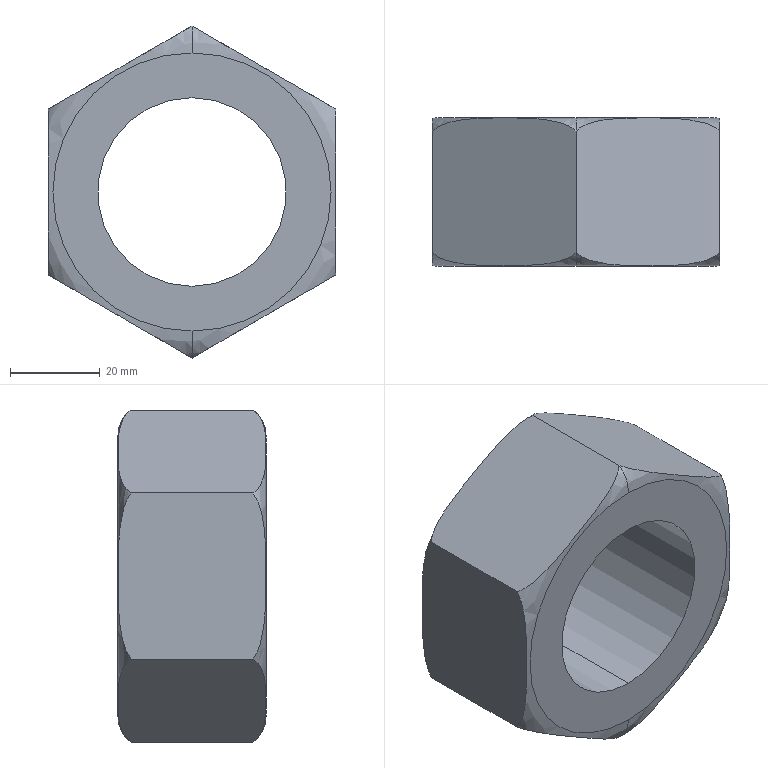Part | SolidWorks | features Extrusion 1, RevCut 1 | 1 solid | 14 faces | box 64 x 33 x 73.901 mm | volume 71017 mm3 | plane 8 | spline 4 | cylinder 2 | commonest cylinder face diameters 42 x2
STEP:
#1=CARTESIAN_POINT('',(0.,13.5,-36.95));
#2=VERTEX_POINT('',#1);
#3=CARTESIAN_POINT('',(32.,13.5,-18.475));
#4=VERTEX_POINT('',#3);
#5=CARTESIAN_POINT('',(0.,13.5,-36.95));
#6=CARTESIAN_POINT('',(0.5345,14.021,-36.642));
#7=CARTESIAN_POINT('',(1.133,14.41,-36.297));
#8=CARTESIAN_POINT('',(2.082,14.885,-35.749));
#9=CARTESIAN_POINT('',(2.409,15.025,-35.56));
#10=CARTESIAN_POINT('',(3.065,15.271,-35.181));
#11=CARTESIAN_POINT('',(3.395,15.377,-34.99));
#12=CARTESIAN_POINT('',(4.392,15.661,-34.414));
#13=CARTESIAN_POINT('',(5.064,15.802,-34.026));
#14=CARTESIAN_POINT('',(6.417,16.026,-33.246));
#15=CARTESIAN_POINT('',(7.097,16.109,-32.853));
#16=CARTESIAN_POINT('',(8.464,16.239,-32.064));
#17=CARTESIAN_POINT('',(9.15,16.285,-31.668));
#18=CARTESIAN_POINT('',(10.522,16.356,-30.876));
#19=CARTESIAN_POINT('',(11.207,16.38,-30.48));
#20=CARTESIAN_POINT('',(13.265,16.433,-29.292));
#21=CARTESIAN_POINT('',(14.637,16.443,-28.5));
#22=CARTESIAN_POINT('',(17.381,16.443,-26.915));
#23=CARTESIAN_POINT('',(18.753,16.432,-26.123));
#24=CARTESIAN_POINT('',(21.498,16.362,-24.538));
#25=CARTESIAN_POINT('',(22.87,16.303,-23.747));
#26=CARTESIAN_POINT('',(24.92,16.107,-22.563));
#27=CARTESIAN_POINT('',(25.603,16.023,-22.169));
#28=CARTESIAN_POINT('',(26.963,15.796,-21.383));
#29=CARTESIAN_POINT('',(27.638,15.654,-20.994));
#30=CARTESIAN_POINT('',(28.969,15.272,-20.225));
#31=CARTESIAN_POINT('',(29.629,15.031,-19.844));
#32=CARTESIAN_POINT('',(30.564,14.561,-19.304));
#33=CARTESIAN_POINT('',(30.868,14.385,-19.129));
#34=CARTESIAN_POINT('',(31.452,13.984,-18.791));
#35=CARTESIAN_POINT('',(31.734,13.759,-18.629));
#36=CARTESIAN_POINT('',(32.,13.5,-18.475));
#37=B_SPLINE_CURVE_WITH_KNOTS('',3,(#5,#6,#7,#8,#9,#10,#11,#12,#13,#14,#15,#16,#17,#18,#19,#20,#21,#22,#23,#24,#25,#26,#27,#28,#29,#30,#31,#32,#33,#34,#35,#36),.UNSPECIFIED.,.F.,.F.,(4,2,2,2,2,2,2,2,2,2,2,2,2,2,2,4),(0.,0.002378,0.003566,0.004755,0.007133,0.009511,0.01189,0.01427,0.01902,0.02378,0.02853,0.03091,0.03329,0.03566,0.03685,0.03804),.UNSPECIFIED.);
#38=EDGE_CURVE('',#2,#4,#37,.T.);
#39=ORIENTED_EDGE('',*,*,#38,.F.);
#40=CARTESIAN_POINT('',(0.,16.5,-30.95));
#41=VERTEX_POINT('',#40);
#42=CARTESIAN_POINT('',(0.,13.5,-36.95));
#43=CARTESIAN_POINT('',(0.,15.629,-35.689));
#44=CARTESIAN_POINT('',(0.,16.5,-33.372));
#45=CARTESIAN_POINT('',(0.,16.5,-30.95));
#46=B_SPLINE_CURVE_WITH_KNOTS('',3,(#42,#43,#44,#45),.UNSPECIFIED.,.F.,.F.,(4,4),(0.,1.),.UNSPECIFIED.);
#47=EDGE_CURVE('',#2,#41,#46,.T.);
#48=ORIENTED_EDGE('',*,*,#47,.T.);
#49=CARTESIAN_POINT('',(0.,16.5,30.95));
#50=VERTEX_POINT('',#49);
#51=CARTESIAN_POINT('',(0.,16.5,0.));
#52=DIRECTION('',(0.,1.,0.));
#53=DIRECTION('',(0.,0.,1.));
#54=AXIS2_PLACEMENT_3D('',#51,#52,#53);
#55=CIRCLE('',#54,30.95);
#56=EDGE_CURVE('',#50,#41,#55,.T.);
#57=ORIENTED_EDGE('',*,*,#56,.F.);
#58=CARTESIAN_POINT('',(0.,13.5,36.95));
#59=VERTEX_POINT('',#58);
#60=CARTESIAN_POINT('',(0.,13.5,36.95));
#61=CARTESIAN_POINT('',(0.,15.629,35.689));
#62=CARTESIAN_POINT('',(0.,16.5,33.372));
#63=CARTESIAN_POINT('',(0.,16.5,30.95));
#64=B_SPLINE_CURVE_WITH_KNOTS('',3,(#60,#61,#62,#63),.UNSPECIFIED.,.F.,.F.,(4,4),(0.,1.),.UNSPECIFIED.);
#65=EDGE_CURVE('',#59,#50,#64,.T.);
#66=ORIENTED_EDGE('',*,*,#65,.F.);
#67=CARTESIAN_POINT('',(32.,13.5,18.475));
#68=VERTEX_POINT('',#67);
#69=CARTESIAN_POINT('',(32.,13.5,18.475));
#70=CARTESIAN_POINT('',(31.465,14.021,18.784));
#71=CARTESIAN_POINT('',(30.867,14.41,19.129));
#72=CARTESIAN_POINT('',(29.918,14.885,19.677));
#73=CARTESIAN_POINT('',(29.591,15.025,19.866));
#74=CARTESIAN_POINT('',(28.935,15.271,20.245));
#75=CARTESIAN_POINT('',(28.605,15.377,20.436));
#76=CARTESIAN_POINT('',(27.608,15.661,21.011));
#77=CARTESIAN_POINT('',(26.936,15.802,21.399));
#78=CARTESIAN_POINT('',(25.583,16.026,22.18));
#79=CARTESIAN_POINT('',(24.903,16.109,22.573));
#80=CARTESIAN_POINT('',(23.536,16.239,23.362));
#81=CARTESIAN_POINT('',(22.85,16.285,23.758));
#82=CARTESIAN_POINT('',(21.478,16.356,24.55));
#83=CARTESIAN_POINT('',(20.793,16.38,24.946));
#84=CARTESIAN_POINT('',(18.735,16.433,26.134));
#85=CARTESIAN_POINT('',(17.363,16.443,26.926));
#86=CARTESIAN_POINT('',(14.619,16.443,28.51));
#87=CARTESIAN_POINT('',(13.247,16.432,29.303));
#88=CARTESIAN_POINT('',(10.502,16.362,30.887));
#89=CARTESIAN_POINT('',(9.13,16.303,31.679));
#90=CARTESIAN_POINT('',(7.08,16.107,32.863));
#91=CARTESIAN_POINT('',(6.397,16.023,33.257));
#92=CARTESIAN_POINT('',(5.037,15.796,34.042));
#93=CARTESIAN_POINT('',(4.362,15.654,34.432));
#94=CARTESIAN_POINT('',(3.031,15.272,35.201));
#95=CARTESIAN_POINT('',(2.371,15.031,35.582));
#96=CARTESIAN_POINT('',(1.436,14.561,36.122));
#97=CARTESIAN_POINT('',(1.132,14.385,36.297));
#98=CARTESIAN_POINT('',(0.5476,13.984,36.634));
#99=CARTESIAN_POINT('',(0.2662,13.759,36.797));
#100=CARTESIAN_POINT('',(0.,13.5,36.95));
#101=B_SPLINE_CURVE_WITH_KNOTS('',3,(#69,#70,#71,#72,#73,#74,#75,#76,#77,#78,#79,#80,#81,#82,#83,#84,#85,#86,#87,#88,#89,#90,#91,#92,#93,#94,#95,#96,#97,#98,#99,#100),.UNSPECIFIED.,.F.,.F.,(4,2,2,2,2,2,2,2,2,2,2,2,2,2,2,4),(0.,0.002378,0.003566,0.004755,0.007133,0.009511,0.01189,0.01427,0.01902,0.02378,0.02853,0.03091,0.03329,0.03566,0.03685,0.03804),.UNSPECIFIED.);
#102=EDGE_CURVE('',#68,#59,#101,.T.);
#103=ORIENTED_EDGE('',*,*,#102,.F.);
#104=CARTESIAN_POINT('',(32.,13.5,-18.475));
#105=CARTESIAN_POINT('',(32.,14.021,-17.858));
#106=CARTESIAN_POINT('',(32.,14.41,-17.167));
#107=CARTESIAN_POINT('',(32.,14.885,-16.071));
#108=CARTESIAN_POINT('',(32.,15.025,-15.694));
#109=CARTESIAN_POINT('',(32.,15.271,-14.936));
#110=CARTESIAN_POINT('',(32.,15.377,-14.555));
#111=CARTESIAN_POINT('',(32.,15.661,-13.403));
#112=CARTESIAN_POINT('',(32.,15.802,-12.627));
#113=CARTESIAN_POINT('',(32.,16.026,-11.066));
#114=CARTESIAN_POINT('',(32.,16.109,-10.28));
#115=CARTESIAN_POINT('',(32.,16.239,-8.702));
#116=CARTESIAN_POINT('',(32.,16.285,-7.909));
#117=CARTESIAN_POINT('',(32.,16.356,-6.326));
#118=CARTESIAN_POINT('',(32.,16.38,-5.534));
#119=CARTESIAN_POINT('',(32.,16.433,-3.158));
#120=CARTESIAN_POINT('',(32.,16.443,-1.574));
#121=CARTESIAN_POINT('',(32.,16.443,1.595));
#122=CARTESIAN_POINT('',(32.,16.432,3.179));
#123=CARTESIAN_POINT('',(32.,16.362,6.349));
#124=CARTESIAN_POINT('',(32.,16.303,7.932));
#125=CARTESIAN_POINT('',(32.,16.107,10.3));
#126=CARTESIAN_POINT('',(32.,16.023,11.088));
#127=CARTESIAN_POINT('',(32.,15.796,12.659));
#128=CARTESIAN_POINT('',(32.,15.654,13.438));
#129=CARTESIAN_POINT('',(32.,15.272,14.976));
#130=CARTESIAN_POINT('',(32.,15.031,15.738));
#131=CARTESIAN_POINT('',(32.,14.561,16.818));
#132=CARTESIAN_POINT('',(32.,14.385,17.168));
#133=CARTESIAN_POINT('',(32.,13.984,17.843));
#134=CARTESIAN_POINT('',(32.,13.759,18.168));
#135=CARTESIAN_POINT('',(32.,13.5,18.475));
#136=B_SPLINE_CURVE_WITH_KNOTS('',3,(#104,#105,#106,#107,#108,#109,#110,#111,#112,#113,#114,#115,#116,#117,#118,#119,#120,#121,#122,#123,#124,#125,#126,#127,#128,#129,#130,#131,#132,#133,#134,#135),.UNSPECIFIED.,.F.,.F.,(4,2,2,2,2,2,2,2,2,2,2,2,2,2,2,4),(0.,0.002378,0.003566,0.004755,0.007133,0.009511,0.01189,0.01427,0.01902,0.02378,0.02853,0.03091,0.03329,0.03566,0.03685,0.03804),.UNSPECIFIED.);
#137=EDGE_CURVE('',#4,#68,#136,.T.);
#138=ORIENTED_EDGE('',*,*,#137,.F.);
#139=EDGE_LOOP('',(#39,#48,#57,#66,#103,#138));
#140=FACE_OUTER_BOUND('',#139,.T.);
#141=CARTESIAN_POINT('',(0.,13.5,36.95));
#142=CARTESIAN_POINT('',(73.901,13.5,36.95));
#143=CARTESIAN_POINT('',(73.901,13.5,-36.95));
#144=CARTESIAN_POINT('',(0.,13.5,-36.95));
#145=CARTESIAN_POINT('',(0.,15.629,35.689));
#146=CARTESIAN_POINT('',(71.378,15.629,35.689));
#147=CARTESIAN_POINT('',(71.378,15.629,-35.689));
#148=CARTESIAN_POINT('',(0.,15.629,-35.689));
#149=CARTESIAN_POINT('',(0.,16.5,33.372));
#150=CARTESIAN_POINT('',(66.744,16.5,33.372));
#151=CARTESIAN_POINT('',(66.744,16.5,-33.372));
#152=CARTESIAN_POINT('',(0.,16.5,-33.372));
#153=CARTESIAN_POINT('',(0.,16.5,30.95));
#154=CARTESIAN_POINT('',(61.901,16.5,30.95));
#155=CARTESIAN_POINT('',(61.901,16.5,-30.95));
#156=CARTESIAN_POINT('',(0.,16.5,-30.95));
#157=(BOUNDED_SURFACE()B_SPLINE_SURFACE(3,3,((#141,#142,#143,#144),(#145,#146,#147,#148),(#149,#150,#151,#152),(#153,#154,#155,#156)),.UNSPECIFIED.,.F.,.F.,.F.)B_SPLINE_SURFACE_WITH_KNOTS((4,4),(4,4),(0.,1.),(0.,1.),.UNSPECIFIED.)GEOMETRIC_REPRESENTATION_ITEM()RATIONAL_B_SPLINE_SURFACE(((1.,0.3333,0.3333,1.),(1.,0.3333,0.3333,1.),(1.,0.3333,0.3333,1.),(1.,0.3333,0.3333,1.)))REPRESENTATION_ITEM('')SURFACE());
#158=ADVANCED_FACE('',(#140),#157,.F.);
#159=CARTESIAN_POINT('',(0.,-16.5,30.95));
#160=VERTEX_POINT('',#159);
#161=CARTESIAN_POINT('',(0.,-16.5,-30.95));
#162=VERTEX_POINT('',#161);
#163=CARTESIAN_POINT('',(0.,-16.5,0.));
#164=DIRECTION('',(0.,1.,0.));
#165=DIRECTION('',(0.,0.,1.));
#166=AXIS2_PLACEMENT_3D('',#163,#164,#165);
#167=CIRCLE('',#166,30.95);
#168=EDGE_CURVE('',#160,#162,#167,.T.);
#169=ORIENTED_EDGE('',*,*,#168,.T.);
#170=CARTESIAN_POINT('',(0.,-13.5,-36.95));
#171=VERTEX_POINT('',#170);
#172=CARTESIAN_POINT('',(0.,-16.5,-30.95));
#173=CARTESIAN_POINT('',(0.,-16.5,-33.372));
#174=CARTESIAN_POINT('',(0.,-15.629,-35.689));
#175=CARTESIAN_POINT('',(0.,-13.5,-36.95));
#176=B_SPLINE_CURVE_WITH_KNOTS('',3,(#172,#173,#174,#175),.UNSPECIFIED.,.F.,.F.,(4,4),(0.,1.),.UNSPECIFIED.);
#177=EDGE_CURVE('',#162,#171,#176,.T.);
#178=ORIENTED_EDGE('',*,*,#177,.T.);
#179=CARTESIAN_POINT('',(32.,-13.5,-18.475));
#180=VERTEX_POINT('',#179);
#181=CARTESIAN_POINT('',(32.,-13.5,-18.475));
#182=CARTESIAN_POINT('',(31.465,-14.021,-18.784));
#183=CARTESIAN_POINT('',(30.867,-14.41,-19.129));
#184=CARTESIAN_POINT('',(29.918,-14.885,-19.677));
#185=CARTESIAN_POINT('',(29.591,-15.025,-19.866));
#186=CARTESIAN_POINT('',(28.935,-15.271,-20.245));
#187=CARTESIAN_POINT('',(28.605,-15.377,-20.436));
#188=CARTESIAN_POINT('',(27.608,-15.661,-21.011));
#189=CARTESIAN_POINT('',(26.936,-15.802,-21.399));
#190=CARTESIAN_POINT('',(25.583,-16.026,-22.18));
#191=CARTESIAN_POINT('',(24.903,-16.109,-22.573));
#192=CARTESIAN_POINT('',(23.536,-16.239,-23.362));
#193=CARTESIAN_POINT('',(22.85,-16.285,-23.758));
#194=CARTESIAN_POINT('',(21.478,-16.356,-24.55));
#195=CARTESIAN_POINT('',(20.793,-16.38,-24.946));
#196=CARTESIAN_POINT('',(18.735,-16.433,-26.134));
#197=CARTESIAN_POINT('',(17.363,-16.443,-26.926));
#198=CARTESIAN_POINT('',(14.619,-16.443,-28.51));
#199=CARTESIAN_POINT('',(13.247,-16.432,-29.303));
#200=CARTESIAN_POINT('',(10.502,-16.362,-30.887));
#201=CARTESIAN_POINT('',(9.13,-16.303,-31.679));
#202=CARTESIAN_POINT('',(7.08,-16.107,-32.863));
#203=CARTESIAN_POINT('',(6.397,-16.023,-33.257));
#204=CARTESIAN_POINT('',(5.037,-15.796,-34.042));
#205=CARTESIAN_POINT('',(4.362,-15.654,-34.432));
#206=CARTESIAN_POINT('',(3.031,-15.272,-35.201));
#207=CARTESIAN_POINT('',(2.371,-15.031,-35.582));
#208=CARTESIAN_POINT('',(1.436,-14.561,-36.122));
#209=CARTESIAN_POINT('',(1.132,-14.385,-36.297));
#210=CARTESIAN_POINT('',(0.5476,-13.984,-36.634));
#211=CARTESIAN_POINT('',(0.2662,-13.759,-36.797));
#212=CARTESIAN_POINT('',(0.,-13.5,-36.95));
#213=B_SPLINE_CURVE_WITH_KNOTS('',3,(#181,#182,#183,#184,#185,#186,#187,#188,#189,#190,#191,#192,#193,#194,#195,#196,#197,#198,#199,#200,#201,#202,#203,#204,#205,#206,#207,#208,#209,#210,#211,#212),.UNSPECIFIED.,.F.,.F.,(4,2,2,2,2,2,2,2,2,2,2,2,2,2,2,4),(0.,0.002378,0.003566,0.004755,0.007133,0.009511,0.01189,0.01427,0.01902,0.02378,0.02853,0.03091,0.03329,0.03566,0.03685,0.03804),.UNSPECIFIED.);
#214=EDGE_CURVE('',#180,#171,#213,.T.);
#215=ORIENTED_EDGE('',*,*,#214,.F.);
#216=CARTESIAN_POINT('',(32.,-13.5,18.475));
#217=VERTEX_POINT('',#216);
#218=CARTESIAN_POINT('',(32.,-13.5,18.475));
#219=CARTESIAN_POINT('',(32.,-14.021,17.858));
#220=CARTESIAN_POINT('',(32.,-14.41,17.167));
#221=CARTESIAN_POINT('',(32.,-14.885,16.071));
#222=CARTESIAN_POINT('',(32.,-15.025,15.694));
#223=CARTESIAN_POINT('',(32.,-15.271,14.936));
#224=CARTESIAN_POINT('',(32.,-15.377,14.555));
#225=CARTESIAN_POINT('',(32.,-15.661,13.403));
#226=CARTESIAN_POINT('',(32.,-15.802,12.627));
#227=CARTESIAN_POINT('',(32.,-16.026,11.066));
#228=CARTESIAN_POINT('',(32.,-16.109,10.28));
#229=CARTESIAN_POINT('',(32.,-16.239,8.702));
#230=CARTESIAN_POINT('',(32.,-16.285,7.909));
#231=CARTESIAN_POINT('',(32.,-16.356,6.326));
#232=CARTESIAN_POINT('',(32.,-16.38,5.534));
#233=CARTESIAN_POINT('',(32.,-16.433,3.158));
#234=CARTESIAN_POINT('',(32.,-16.443,1.574));
#235=CARTESIAN_POINT('',(32.,-16.443,-1.595));
#236=CARTESIAN_POINT('',(32.,-16.432,-3.179));
#237=CARTESIAN_POINT('',(32.,-16.362,-6.349));
#238=CARTESIAN_POINT('',(32.,-16.303,-7.932));
#239=CARTESIAN_POINT('',(32.,-16.107,-10.3));
#240=CARTESIAN_POINT('',(32.,-16.023,-11.088));
#241=CARTESIAN_POINT('',(32.,-15.796,-12.659));
#242=CARTESIAN_POINT('',(32.,-15.654,-13.438));
#243=CARTESIAN_POINT('',(32.,-15.272,-14.976));
#244=CARTESIAN_POINT('',(32.,-15.031,-15.738));
#245=CARTESIAN_POINT('',(32.,-14.561,-16.818));
#246=CARTESIAN_POINT('',(32.,-14.385,-17.168));
#247=CARTESIAN_POINT('',(32.,-13.984,-17.843));
#248=CARTESIAN_POINT('',(32.,-13.759,-18.168));
#249=CARTESIAN_POINT('',(32.,-13.5,-18.475));
#250=B_SPLINE_CURVE_WITH_KNOTS('',3,(#218,#219,#220,#221,#222,#223,#224,#225,#226,#227,#228,#229,#230,#231,#232,#233,#234,#235,#236,#237,#238,#239,#240,#241,#242,#243,#244,#245,#246,#247,#248,#249),.UNSPECIFIED.,.F.,.F.,(4,2,2,2,2,2,2,2,2,2,2,2,2,2,2,4),(0.,0.002378,0.003566,0.004755,0.007133,0.009511,0.01189,0.01427,0.01902,0.02378,0.02853,0.03091,0.03329,0.03566,0.03685,0.03804),.UNSPECIFIED.);
#251=EDGE_CURVE('',#217,#180,#250,.T.);
#252=ORIENTED_EDGE('',*,*,#251,.F.);
#253=CARTESIAN_POINT('',(0.,-13.5,36.95));
#254=VERTEX_POINT('',#253);
#255=CARTESIAN_POINT('',(0.,-13.5,36.95));
#256=CARTESIAN_POINT('',(0.5345,-14.021,36.642));
#257=CARTESIAN_POINT('',(1.133,-14.41,36.297));
#258=CARTESIAN_POINT('',(2.082,-14.885,35.749));
#259=CARTESIAN_POINT('',(2.409,-15.025,35.56));
#260=CARTESIAN_POINT('',(3.065,-15.271,35.181));
#261=CARTESIAN_POINT('',(3.395,-15.377,34.99));
#262=CARTESIAN_POINT('',(4.392,-15.661,34.414));
#263=CARTESIAN_POINT('',(5.064,-15.802,34.026));
#264=CARTESIAN_POINT('',(6.417,-16.026,33.246));
#265=CARTESIAN_POINT('',(7.097,-16.109,32.853));
#266=CARTESIAN_POINT('',(8.464,-16.239,32.064));
#267=CARTESIAN_POINT('',(9.15,-16.285,31.668));
#268=CARTESIAN_POINT('',(10.522,-16.356,30.876));
#269=CARTESIAN_POINT('',(11.207,-16.38,30.48));
#270=CARTESIAN_POINT('',(13.265,-16.433,29.292));
#271=CARTESIAN_POINT('',(14.637,-16.443,28.5));
#272=CARTESIAN_POINT('',(17.381,-16.443,26.915));
#273=CARTESIAN_POINT('',(18.753,-16.432,26.123));
#274=CARTESIAN_POINT('',(21.498,-16.362,24.538));
#275=CARTESIAN_POINT('',(22.87,-16.303,23.747));
#276=CARTESIAN_POINT('',(24.92,-16.107,22.563));
#277=CARTESIAN_POINT('',(25.603,-16.023,22.169));
#278=CARTESIAN_POINT('',(26.963,-15.796,21.383));
#279=CARTESIAN_POINT('',(27.638,-15.654,20.994));
#280=CARTESIAN_POINT('',(28.969,-15.272,20.225));
#281=CARTESIAN_POINT('',(29.629,-15.031,19.844));
#282=CARTESIAN_POINT('',(30.564,-14.561,19.304));
#283=CARTESIAN_POINT('',(30.868,-14.385,19.129));
#284=CARTESIAN_POINT('',(31.452,-13.984,18.791));
#285=CARTESIAN_POINT('',(31.734,-13.759,18.629));
#286=CARTESIAN_POINT('',(32.,-13.5,18.475));
#287=B_SPLINE_CURVE_WITH_KNOTS('',3,(#255,#256,#257,#258,#259,#260,#261,#262,#263,#264,#265,#266,#267,#268,#269,#270,#271,#272,#273,#274,#275,#276,#277,#278,#279,#280,#281,#282,#283,#284,#285,#286),.UNSPECIFIED.,.F.,.F.,(4,2,2,2,2,2,2,2,2,2,2,2,2,2,2,4),(0.,0.002378,0.003566,0.004755,0.007133,0.009511,0.01189,0.01427,0.01902,0.02378,0.02853,0.03091,0.03329,0.03566,0.03685,0.03804),.UNSPECIFIED.);
#288=EDGE_CURVE('',#254,#217,#287,.T.);
#289=ORIENTED_EDGE('',*,*,#288,.F.);
#290=CARTESIAN_POINT('',(0.,-16.5,30.95));
#291=CARTESIAN_POINT('',(0.,-16.5,33.372));
#292=CARTESIAN_POINT('',(0.,-15.629,35.689));
#293=CARTESIAN_POINT('',(0.,-13.5,36.95));
#294=B_SPLINE_CURVE_WITH_KNOTS('',3,(#290,#291,#292,#293),.UNSPECIFIED.,.F.,.F.,(4,4),(0.,1.),.UNSPECIFIED.);
#295=EDGE_CURVE('',#160,#254,#294,.T.);
#296=ORIENTED_EDGE('',*,*,#295,.F.);
#297=EDGE_LOOP('',(#169,#178,#215,#252,#289,#296));
#298=FACE_OUTER_BOUND('',#297,.T.);
#299=CARTESIAN_POINT('',(0.,-16.5,30.95));
#300=CARTESIAN_POINT('',(61.901,-16.5,30.95));
#301=CARTESIAN_POINT('',(61.901,-16.5,-30.95));
#302=CARTESIAN_POINT('',(0.,-16.5,-30.95));
#303=CARTESIAN_POINT('',(0.,-16.5,33.372));
#304=CARTESIAN_POINT('',(66.744,-16.5,33.372));
#305=CARTESIAN_POINT('',(66.744,-16.5,-33.372));
#306=CARTESIAN_POINT('',(0.,-16.5,-33.372));
#307=CARTESIAN_POINT('',(0.,-15.629,35.689));
#308=CARTESIAN_POINT('',(71.378,-15.629,35.689));
#309=CARTESIAN_POINT('',(71.378,-15.629,-35.689));
#310=CARTESIAN_POINT('',(0.,-15.629,-35.689));
#311=CARTESIAN_POINT('',(0.,-13.5,36.95));
#312=CARTESIAN_POINT('',(73.901,-13.5,36.95));
#313=CARTESIAN_POINT('',(73.901,-13.5,-36.95));
#314=CARTESIAN_POINT('',(0.,-13.5,-36.95));
#315=(BOUNDED_SURFACE()B_SPLINE_SURFACE(3,3,((#299,#300,#301,#302),(#303,#304,#305,#306),(#307,#308,#309,#310),(#311,#312,#313,#314)),.UNSPECIFIED.,.F.,.F.,.F.)B_SPLINE_SURFACE_WITH_KNOTS((4,4),(4,4),(0.,1.),(0.,1.),.UNSPECIFIED.)GEOMETRIC_REPRESENTATION_ITEM()RATIONAL_B_SPLINE_SURFACE(((1.,0.3333,0.3333,1.),(1.,0.3333,0.3333,1.),(1.,0.3333,0.3333,1.),(1.,0.3333,0.3333,1.)))REPRESENTATION_ITEM('')SURFACE());
#316=ADVANCED_FACE('',(#298),#315,.F.);
#317=CARTESIAN_POINT('',(0.,16.5,-21.));
#318=VERTEX_POINT('',#317);
#319=CARTESIAN_POINT('',(0.,16.5,21.));
#320=VERTEX_POINT('',#319);
#321=CARTESIAN_POINT('',(0.,16.5,0.));
#322=DIRECTION('',(0.,1.,0.));
#323=DIRECTION('',(0.,0.,1.));
#324=AXIS2_PLACEMENT_3D('',#321,#322,#323);
#325=CIRCLE('',#324,21.);
#326=EDGE_CURVE('',#318,#320,#325,.T.);
#327=ORIENTED_EDGE('',*,*,#326,.T.);
#328=CARTESIAN_POINT('',(0.,-16.5,21.));
#329=VERTEX_POINT('',#328);
#330=CARTESIAN_POINT('',(0.,16.5,21.));
#331=DIRECTION('',(0.,-1.,0.));
#332=VECTOR('',#331,1000.);
#333=LINE('',#330,#332);
#334=EDGE_CURVE('',#320,#329,#333,.T.);
#335=ORIENTED_EDGE('',*,*,#334,.T.);
#336=CARTESIAN_POINT('',(0.,-16.5,-21.));
#337=VERTEX_POINT('',#336);
#338=CARTESIAN_POINT('',(0.,-16.5,0.));
#339=DIRECTION('',(0.,1.,0.));
#340=DIRECTION('',(0.,0.,1.));
#341=AXIS2_PLACEMENT_3D('',#338,#339,#340);
#342=CIRCLE('',#341,21.);
#343=EDGE_CURVE('',#337,#329,#342,.T.);
#344=ORIENTED_EDGE('',*,*,#343,.F.);
#345=CARTESIAN_POINT('',(0.,16.5,-21.));
#346=DIRECTION('',(0.,-1.,0.));
#347=VECTOR('',#346,1000.);
#348=LINE('',#345,#347);
#349=EDGE_CURVE('',#318,#337,#348,.T.);
#350=ORIENTED_EDGE('',*,*,#349,.F.);
#351=EDGE_LOOP('',(#327,#335,#344,#350));
#352=FACE_OUTER_BOUND('',#351,.T.);
#353=CARTESIAN_POINT('',(0.,16.5,0.));
#354=DIRECTION('',(0.,-1.,0.));
#355=DIRECTION('',(0.,0.,-1.));
#356=AXIS2_PLACEMENT_3D('',#353,#354,#355);
#357=CYLINDRICAL_SURFACE('',#356,21.);
#358=ADVANCED_FACE('',(#352),#357,.F.);
#359=ORIENTED_EDGE('',*,*,#326,.F.);
#360=CARTESIAN_POINT('',(0.,16.5,0.));
#361=DIRECTION('',(0.,1.,0.));
#362=DIRECTION('',(0.,0.,1.));
#363=AXIS2_PLACEMENT_3D('',#360,#361,#362);
#364=CIRCLE('',#363,21.);
#365=EDGE_CURVE('',#320,#318,#364,.T.);
#366=ORIENTED_EDGE('',*,*,#365,.F.);
#367=EDGE_LOOP('',(#359,#366));
#368=FACE_BOUND('',#367,.T.);
#369=ORIENTED_EDGE('',*,*,#56,.T.);
#370=CARTESIAN_POINT('',(0.,16.5,0.));
#371=DIRECTION('',(0.,1.,0.));
#372=DIRECTION('',(0.,0.,1.));
#373=AXIS2_PLACEMENT_3D('',#370,#371,#372);
#374=CIRCLE('',#373,30.95);
#375=EDGE_CURVE('',#41,#50,#374,.T.);
#376=ORIENTED_EDGE('',*,*,#375,.T.);
#377=EDGE_LOOP('',(#369,#376));
#378=FACE_OUTER_BOUND('',#377,.T.);
#379=CARTESIAN_POINT('',(0.,16.5,0.));
#380=DIRECTION('',(0.,1.,0.));
#381=DIRECTION('',(0.,0.,1.));
#382=AXIS2_PLACEMENT_3D('',#379,#380,#381);
#383=PLANE('',#382);
#384=ADVANCED_FACE('',(#368,#378),#383,.T.);
#385=ORIENTED_EDGE('',*,*,#343,.T.);
#386=CARTESIAN_POINT('',(0.,-16.5,0.));
#387=DIRECTION('',(0.,1.,0.));
#388=DIRECTION('',(0.,0.,1.));
#389=AXIS2_PLACEMENT_3D('',#386,#387,#388);
#390=CIRCLE('',#389,21.);
#391=EDGE_CURVE('',#329,#337,#390,.T.);
#392=ORIENTED_EDGE('',*,*,#391,.T.);
#393=EDGE_LOOP('',(#385,#392));
#394=FACE_BOUND('',#393,.T.);
#395=ORIENTED_EDGE('',*,*,#168,.F.);
#396=CARTESIAN_POINT('',(0.,-16.5,0.));
#397=DIRECTION('',(0.,1.,0.));
#398=DIRECTION('',(0.,0.,1.));
#399=AXIS2_PLACEMENT_3D('',#396,#397,#398);
#400=CIRCLE('',#399,30.95);
#401=EDGE_CURVE('',#162,#160,#400,.T.);
#402=ORIENTED_EDGE('',*,*,#401,.F.);
#403=EDGE_LOOP('',(#395,#402));
#404=FACE_OUTER_BOUND('',#403,.T.);
#405=CARTESIAN_POINT('',(0.,-16.5,0.));
#406=DIRECTION('',(0.,1.,0.));
#407=DIRECTION('',(0.,0.,1.));
#408=AXIS2_PLACEMENT_3D('',#405,#406,#407);
#409=PLANE('',#408);
#410=ADVANCED_FACE('',(#394,#404),#409,.F.);
#411=ORIENTED_EDGE('',*,*,#334,.F.);
#412=ORIENTED_EDGE('',*,*,#365,.T.);
#413=ORIENTED_EDGE('',*,*,#349,.T.);
#414=ORIENTED_EDGE('',*,*,#391,.F.);
#415=EDGE_LOOP('',(#411,#412,#413,#414));
#416=FACE_OUTER_BOUND('',#415,.T.);
#417=CARTESIAN_POINT('',(0.,16.5,0.));
#418=DIRECTION('',(0.,-1.,0.));
#419=DIRECTION('',(0.,0.,-1.));
#420=AXIS2_PLACEMENT_3D('',#417,#418,#419);
#421=CYLINDRICAL_SURFACE('',#420,21.);
#422=ADVANCED_FACE('',(#416),#421,.F.);
#423=ORIENTED_EDGE('',*,*,#177,.F.);
#424=ORIENTED_EDGE('',*,*,#401,.T.);
#425=ORIENTED_EDGE('',*,*,#295,.T.);
#426=CARTESIAN_POINT('',(-32.,-13.5,18.475));
#427=VERTEX_POINT('',#426);
#428=CARTESIAN_POINT('',(-32.,-13.5,18.475));
#429=CARTESIAN_POINT('',(-31.465,-14.021,18.784));
#430=CARTESIAN_POINT('',(-30.867,-14.41,19.129));
#431=CARTESIAN_POINT('',(-29.918,-14.885,19.677));
#432=CARTESIAN_POINT('',(-29.591,-15.025,19.866));
#433=CARTESIAN_POINT('',(-28.935,-15.271,20.245));
#434=CARTESIAN_POINT('',(-28.605,-15.377,20.436));
#435=CARTESIAN_POINT('',(-27.608,-15.661,21.011));
#436=CARTESIAN_POINT('',(-26.936,-15.802,21.399));
#437=CARTESIAN_POINT('',(-25.583,-16.026,22.18));
#438=CARTESIAN_POINT('',(-24.903,-16.109,22.573));
#439=CARTESIAN_POINT('',(-23.536,-16.239,23.362));
#440=CARTESIAN_POINT('',(-22.85,-16.285,23.758));
#441=CARTESIAN_POINT('',(-21.478,-16.356,24.55));
#442=CARTESIAN_POINT('',(-20.793,-16.38,24.946));
#443=CARTESIAN_POINT('',(-18.735,-16.433,26.134));
#444=CARTESIAN_POINT('',(-17.363,-16.443,26.926));
#445=CARTESIAN_POINT('',(-14.619,-16.443,28.51));
#446=CARTESIAN_POINT('',(-13.247,-16.432,29.303));
#447=CARTESIAN_POINT('',(-10.502,-16.362,30.887));
#448=CARTESIAN_POINT('',(-9.13,-16.303,31.679));
#449=CARTESIAN_POINT('',(-7.08,-16.107,32.863));
#450=CARTESIAN_POINT('',(-6.397,-16.023,33.257));
#451=CARTESIAN_POINT('',(-5.037,-15.796,34.042));
#452=CARTESIAN_POINT('',(-4.362,-15.654,34.432));
#453=CARTESIAN_POINT('',(-3.031,-15.272,35.201));
#454=CARTESIAN_POINT('',(-2.371,-15.031,35.582));
#455=CARTESIAN_POINT('',(-1.436,-14.561,36.122));
#456=CARTESIAN_POINT('',(-1.132,-14.385,36.297));
#457=CARTESIAN_POINT('',(-0.5476,-13.984,36.634));
#458=CARTESIAN_POINT('',(-0.2662,-13.759,36.797));
#459=CARTESIAN_POINT('',(0.,-13.5,36.95));
#460=B_SPLINE_CURVE_WITH_KNOTS('',3,(#428,#429,#430,#431,#432,#433,#434,#435,#436,#437,#438,#439,#440,#441,#442,#443,#444,#445,#446,#447,#448,#449,#450,#451,#452,#453,#454,#455,#456,#457,#458,#459),.UNSPECIFIED.,.F.,.F.,(4,2,2,2,2,2,2,2,2,2,2,2,2,2,2,4),(0.,0.002378,0.003566,0.004755,0.007133,0.009511,0.01189,0.01427,0.01902,0.02378,0.02853,0.03091,0.03329,0.03566,0.03685,0.03804),.UNSPECIFIED.);
#461=EDGE_CURVE('',#427,#254,#460,.T.);
#462=ORIENTED_EDGE('',*,*,#461,.F.);
#463=CARTESIAN_POINT('',(-32.,-13.5,-18.475));
#464=VERTEX_POINT('',#463);
#465=CARTESIAN_POINT('',(-32.,-13.5,-18.475));
#466=CARTESIAN_POINT('',(-32.,-14.021,-17.858));
#467=CARTESIAN_POINT('',(-32.,-14.41,-17.167));
#468=CARTESIAN_POINT('',(-32.,-14.885,-16.071));
#469=CARTESIAN_POINT('',(-32.,-15.025,-15.694));
#470=CARTESIAN_POINT('',(-32.,-15.271,-14.936));
#471=CARTESIAN_POINT('',(-32.,-15.377,-14.555));
#472=CARTESIAN_POINT('',(-32.,-15.661,-13.403));
#473=CARTESIAN_POINT('',(-32.,-15.802,-12.627));
#474=CARTESIAN_POINT('',(-32.,-16.026,-11.066));
#475=CARTESIAN_POINT('',(-32.,-16.109,-10.28));
#476=CARTESIAN_POINT('',(-32.,-16.239,-8.702));
#477=CARTESIAN_POINT('',(-32.,-16.285,-7.909));
#478=CARTESIAN_POINT('',(-32.,-16.356,-6.326));
#479=CARTESIAN_POINT('',(-32.,-16.38,-5.534));
#480=CARTESIAN_POINT('',(-32.,-16.433,-3.158));
#481=CARTESIAN_POINT('',(-32.,-16.443,-1.574));
#482=CARTESIAN_POINT('',(-32.,-16.443,1.595));
#483=CARTESIAN_POINT('',(-32.,-16.432,3.179));
#484=CARTESIAN_POINT('',(-32.,-16.362,6.349));
#485=CARTESIAN_POINT('',(-32.,-16.303,7.932));
#486=CARTESIAN_POINT('',(-32.,-16.107,10.3));
#487=CARTESIAN_POINT('',(-32.,-16.023,11.088));
#488=CARTESIAN_POINT('',(-32.,-15.796,12.659));
#489=CARTESIAN_POINT('',(-32.,-15.654,13.438));
#490=CARTESIAN_POINT('',(-32.,-15.272,14.976));
#491=CARTESIAN_POINT('',(-32.,-15.031,15.738));
#492=CARTESIAN_POINT('',(-32.,-14.561,16.818));
#493=CARTESIAN_POINT('',(-32.,-14.385,17.168));
#494=CARTESIAN_POINT('',(-32.,-13.984,17.843));
#495=CARTESIAN_POINT('',(-32.,-13.759,18.168));
#496=CARTESIAN_POINT('',(-32.,-13.5,18.475));
#497=B_SPLINE_CURVE_WITH_KNOTS('',3,(#465,#466,#467,#468,#469,#470,#471,#472,#473,#474,#475,#476,#477,#478,#479,#480,#481,#482,#483,#484,#485,#486,#487,#488,#489,#490,#491,#492,#493,#494,#495,#496),.UNSPECIFIED.,.F.,.F.,(4,2,2,2,2,2,2,2,2,2,2,2,2,2,2,4),(0.,0.002378,0.003566,0.004755,0.007133,0.009511,0.01189,0.01427,0.01902,0.02378,0.02853,0.03091,0.03329,0.03566,0.03685,0.03804),.UNSPECIFIED.);
#498=EDGE_CURVE('',#464,#427,#497,.T.);
#499=ORIENTED_EDGE('',*,*,#498,.F.);
#500=CARTESIAN_POINT('',(0.,-13.5,-36.95));
#501=CARTESIAN_POINT('',(-0.5345,-14.021,-36.642));
#502=CARTESIAN_POINT('',(-1.133,-14.41,-36.297));
#503=CARTESIAN_POINT('',(-2.082,-14.885,-35.749));
#504=CARTESIAN_POINT('',(-2.409,-15.025,-35.56));
#505=CARTESIAN_POINT('',(-3.065,-15.271,-35.181));
#506=CARTESIAN_POINT('',(-3.395,-15.377,-34.99));
#507=CARTESIAN_POINT('',(-4.392,-15.661,-34.414));
#508=CARTESIAN_POINT('',(-5.064,-15.802,-34.026));
#509=CARTESIAN_POINT('',(-6.417,-16.026,-33.246));
#510=CARTESIAN_POINT('',(-7.097,-16.109,-32.853));
#511=CARTESIAN_POINT('',(-8.464,-16.239,-32.064));
#512=CARTESIAN_POINT('',(-9.15,-16.285,-31.668));
#513=CARTESIAN_POINT('',(-10.522,-16.356,-30.876));
#514=CARTESIAN_POINT('',(-11.207,-16.38,-30.48));
#515=CARTESIAN_POINT('',(-13.265,-16.433,-29.292));
#516=CARTESIAN_POINT('',(-14.637,-16.443,-28.5));
#517=CARTESIAN_POINT('',(-17.381,-16.443,-26.915));
#518=CARTESIAN_POINT('',(-18.753,-16.432,-26.123));
#519=CARTESIAN_POINT('',(-21.498,-16.362,-24.538));
#520=CARTESIAN_POINT('',(-22.87,-16.303,-23.747));
#521=CARTESIAN_POINT('',(-24.92,-16.107,-22.563));
#522=CARTESIAN_POINT('',(-25.603,-16.023,-22.169));
#523=CARTESIAN_POINT('',(-26.963,-15.796,-21.383));
#524=CARTESIAN_POINT('',(-27.638,-15.654,-20.994));
#525=CARTESIAN_POINT('',(-28.969,-15.272,-20.225));
#526=CARTESIAN_POINT('',(-29.629,-15.031,-19.844));
#527=CARTESIAN_POINT('',(-30.564,-14.561,-19.304));
#528=CARTESIAN_POINT('',(-30.868,-14.385,-19.129));
#529=CARTESIAN_POINT('',(-31.452,-13.984,-18.791));
#530=CARTESIAN_POINT('',(-31.734,-13.759,-18.629));
#531=CARTESIAN_POINT('',(-32.,-13.5,-18.475));
#532=B_SPLINE_CURVE_WITH_KNOTS('',3,(#500,#501,#502,#503,#504,#505,#506,#507,#508,#509,#510,#511,#512,#513,#514,#515,#516,#517,#518,#519,#520,#521,#522,#523,#524,#525,#526,#527,#528,#529,#530,#531),.UNSPECIFIED.,.F.,.F.,(4,2,2,2,2,2,2,2,2,2,2,2,2,2,2,4),(0.,0.002378,0.003566,0.004755,0.007133,0.009511,0.01189,0.01427,0.01902,0.02378,0.02853,0.03091,0.03329,0.03566,0.03685,0.03804),.UNSPECIFIED.);
#533=EDGE_CURVE('',#171,#464,#532,.T.);
#534=ORIENTED_EDGE('',*,*,#533,.F.);
#535=EDGE_LOOP('',(#423,#424,#425,#462,#499,#534));
#536=FACE_OUTER_BOUND('',#535,.T.);
#537=CARTESIAN_POINT('',(0.,-16.5,-30.95));
#538=CARTESIAN_POINT('',(-61.901,-16.5,-30.95));
#539=CARTESIAN_POINT('',(-61.901,-16.5,30.95));
#540=CARTESIAN_POINT('',(0.,-16.5,30.95));
#541=CARTESIAN_POINT('',(0.,-16.5,-33.372));
#542=CARTESIAN_POINT('',(-66.744,-16.5,-33.372));
#543=CARTESIAN_POINT('',(-66.744,-16.5,33.372));
#544=CARTESIAN_POINT('',(0.,-16.5,33.372));
#545=CARTESIAN_POINT('',(0.,-15.629,-35.689));
#546=CARTESIAN_POINT('',(-71.378,-15.629,-35.689));
#547=CARTESIAN_POINT('',(-71.378,-15.629,35.689));
#548=CARTESIAN_POINT('',(0.,-15.629,35.689));
#549=CARTESIAN_POINT('',(0.,-13.5,-36.95));
#550=CARTESIAN_POINT('',(-73.901,-13.5,-36.95));
#551=CARTESIAN_POINT('',(-73.901,-13.5,36.95));
#552=CARTESIAN_POINT('',(0.,-13.5,36.95));
#553=(BOUNDED_SURFACE()B_SPLINE_SURFACE(3,3,((#537,#538,#539,#540),(#541,#542,#543,#544),(#545,#546,#547,#548),(#549,#550,#551,#552)),.UNSPECIFIED.,.F.,.F.,.F.)B_SPLINE_SURFACE_WITH_KNOTS((4,4),(4,4),(0.,1.),(0.,1.),.UNSPECIFIED.)GEOMETRIC_REPRESENTATION_ITEM()RATIONAL_B_SPLINE_SURFACE(((1.,0.3333,0.3333,1.),(1.,0.3333,0.3333,1.),(1.,0.3333,0.3333,1.),(1.,0.3333,0.3333,1.)))REPRESENTATION_ITEM('')SURFACE());
#554=ADVANCED_FACE('',(#536),#553,.F.);
#555=ORIENTED_EDGE('',*,*,#47,.F.);
#556=CARTESIAN_POINT('',(-32.,13.5,-18.475));
#557=VERTEX_POINT('',#556);
#558=CARTESIAN_POINT('',(-32.,13.5,-18.475));
#559=CARTESIAN_POINT('',(-31.465,14.021,-18.784));
#560=CARTESIAN_POINT('',(-30.867,14.41,-19.129));
#561=CARTESIAN_POINT('',(-29.918,14.885,-19.677));
#562=CARTESIAN_POINT('',(-29.591,15.025,-19.866));
#563=CARTESIAN_POINT('',(-28.935,15.271,-20.245));
#564=CARTESIAN_POINT('',(-28.605,15.377,-20.436));
#565=CARTESIAN_POINT('',(-27.608,15.661,-21.011));
#566=CARTESIAN_POINT('',(-26.936,15.802,-21.399));
#567=CARTESIAN_POINT('',(-25.583,16.026,-22.18));
#568=CARTESIAN_POINT('',(-24.903,16.109,-22.573));
#569=CARTESIAN_POINT('',(-23.536,16.239,-23.362));
#570=CARTESIAN_POINT('',(-22.85,16.285,-23.758));
#571=CARTESIAN_POINT('',(-21.478,16.356,-24.55));
#572=CARTESIAN_POINT('',(-20.793,16.38,-24.946));
#573=CARTESIAN_POINT('',(-18.735,16.433,-26.134));
#574=CARTESIAN_POINT('',(-17.363,16.443,-26.926));
#575=CARTESIAN_POINT('',(-14.619,16.443,-28.51));
#576=CARTESIAN_POINT('',(-13.247,16.432,-29.303));
#577=CARTESIAN_POINT('',(-10.502,16.362,-30.887));
#578=CARTESIAN_POINT('',(-9.13,16.303,-31.679));
#579=CARTESIAN_POINT('',(-7.08,16.107,-32.863));
#580=CARTESIAN_POINT('',(-6.397,16.023,-33.257));
#581=CARTESIAN_POINT('',(-5.037,15.796,-34.042));
#582=CARTESIAN_POINT('',(-4.362,15.654,-34.432));
#583=CARTESIAN_POINT('',(-3.031,15.272,-35.201));
#584=CARTESIAN_POINT('',(-2.371,15.031,-35.582));
#585=CARTESIAN_POINT('',(-1.436,14.561,-36.122));
#586=CARTESIAN_POINT('',(-1.132,14.385,-36.297));
#587=CARTESIAN_POINT('',(-0.5476,13.984,-36.634));
#588=CARTESIAN_POINT('',(-0.2662,13.759,-36.797));
#589=CARTESIAN_POINT('',(0.,13.5,-36.95));
#590=B_SPLINE_CURVE_WITH_KNOTS('',3,(#558,#559,#560,#561,#562,#563,#564,#565,#566,#567,#568,#569,#570,#571,#572,#573,#574,#575,#576,#577,#578,#579,#580,#581,#582,#583,#584,#585,#586,#587,#588,#589),.UNSPECIFIED.,.F.,.F.,(4,2,2,2,2,2,2,2,2,2,2,2,2,2,2,4),(0.,0.002378,0.003566,0.004755,0.007133,0.009511,0.01189,0.01427,0.01902,0.02378,0.02853,0.03091,0.03329,0.03566,0.03685,0.03804),.UNSPECIFIED.);
#591=EDGE_CURVE('',#557,#2,#590,.T.);
#592=ORIENTED_EDGE('',*,*,#591,.F.);
#593=CARTESIAN_POINT('',(-32.,13.5,18.475));
#594=VERTEX_POINT('',#593);
#595=CARTESIAN_POINT('',(-32.,13.5,18.475));
#596=CARTESIAN_POINT('',(-32.,14.021,17.858));
#597=CARTESIAN_POINT('',(-32.,14.41,17.167));
#598=CARTESIAN_POINT('',(-32.,14.885,16.071));
#599=CARTESIAN_POINT('',(-32.,15.025,15.694));
#600=CARTESIAN_POINT('',(-32.,15.271,14.936));
#601=CARTESIAN_POINT('',(-32.,15.377,14.555));
#602=CARTESIAN_POINT('',(-32.,15.661,13.403));
#603=CARTESIAN_POINT('',(-32.,15.802,12.627));
#604=CARTESIAN_POINT('',(-32.,16.026,11.066));
#605=CARTESIAN_POINT('',(-32.,16.109,10.28));
#606=CARTESIAN_POINT('',(-32.,16.239,8.702));
#607=CARTESIAN_POINT('',(-32.,16.285,7.909));
#608=CARTESIAN_POINT('',(-32.,16.356,6.326));
#609=CARTESIAN_POINT('',(-32.,16.38,5.534));
#610=CARTESIAN_POINT('',(-32.,16.433,3.158));
#611=CARTESIAN_POINT('',(-32.,16.443,1.574));
#612=CARTESIAN_POINT('',(-32.,16.443,-1.595));
#613=CARTESIAN_POINT('',(-32.,16.432,-3.179));
#614=CARTESIAN_POINT('',(-32.,16.362,-6.349));
#615=CARTESIAN_POINT('',(-32.,16.303,-7.932));
#616=CARTESIAN_POINT('',(-32.,16.107,-10.3));
#617=CARTESIAN_POINT('',(-32.,16.023,-11.088));
#618=CARTESIAN_POINT('',(-32.,15.796,-12.659));
#619=CARTESIAN_POINT('',(-32.,15.654,-13.438));
#620=CARTESIAN_POINT('',(-32.,15.272,-14.976));
#621=CARTESIAN_POINT('',(-32.,15.031,-15.738));
#622=CARTESIAN_POINT('',(-32.,14.561,-16.818));
#623=CARTESIAN_POINT('',(-32.,14.385,-17.168));
#624=CARTESIAN_POINT('',(-32.,13.984,-17.843));
#625=CARTESIAN_POINT('',(-32.,13.759,-18.168));
#626=CARTESIAN_POINT('',(-32.,13.5,-18.475));
#627=B_SPLINE_CURVE_WITH_KNOTS('',3,(#595,#596,#597,#598,#599,#600,#601,#602,#603,#604,#605,#606,#607,#608,#609,#610,#611,#612,#613,#614,#615,#616,#617,#618,#619,#620,#621,#622,#623,#624,#625,#626),.UNSPECIFIED.,.F.,.F.,(4,2,2,2,2,2,2,2,2,2,2,2,2,2,2,4),(0.,0.002378,0.003566,0.004755,0.007133,0.009511,0.01189,0.01427,0.01902,0.02378,0.02853,0.03091,0.03329,0.03566,0.03685,0.03804),.UNSPECIFIED.);
#628=EDGE_CURVE('',#594,#557,#627,.T.);
#629=ORIENTED_EDGE('',*,*,#628,.F.);
#630=CARTESIAN_POINT('',(0.,13.5,36.95));
#631=CARTESIAN_POINT('',(-0.5345,14.021,36.642));
#632=CARTESIAN_POINT('',(-1.133,14.41,36.297));
#633=CARTESIAN_POINT('',(-2.082,14.885,35.749));
#634=CARTESIAN_POINT('',(-2.409,15.025,35.56));
#635=CARTESIAN_POINT('',(-3.065,15.271,35.181));
#636=CARTESIAN_POINT('',(-3.395,15.377,34.99));
#637=CARTESIAN_POINT('',(-4.392,15.661,34.414));
#638=CARTESIAN_POINT('',(-5.064,15.802,34.026));
#639=CARTESIAN_POINT('',(-6.417,16.026,33.246));
#640=CARTESIAN_POINT('',(-7.097,16.109,32.853));
#641=CARTESIAN_POINT('',(-8.464,16.239,32.064));
#642=CARTESIAN_POINT('',(-9.15,16.285,31.668));
#643=CARTESIAN_POINT('',(-10.522,16.356,30.876));
#644=CARTESIAN_POINT('',(-11.207,16.38,30.48));
#645=CARTESIAN_POINT('',(-13.265,16.433,29.292));
#646=CARTESIAN_POINT('',(-14.637,16.443,28.5));
#647=CARTESIAN_POINT('',(-17.381,16.443,26.915));
#648=CARTESIAN_POINT('',(-18.753,16.432,26.123));
#649=CARTESIAN_POINT('',(-21.498,16.362,24.538));
#650=CARTESIAN_POINT('',(-22.87,16.303,23.747));
#651=CARTESIAN_POINT('',(-24.92,16.107,22.563));
#652=CARTESIAN_POINT('',(-25.603,16.023,22.169));
#653=CARTESIAN_POINT('',(-26.963,15.796,21.383));
#654=CARTESIAN_POINT('',(-27.638,15.654,20.994));
#655=CARTESIAN_POINT('',(-28.969,15.272,20.225));
#656=CARTESIAN_POINT('',(-29.629,15.031,19.844));
#657=CARTESIAN_POINT('',(-30.564,14.561,19.304));
#658=CARTESIAN_POINT('',(-30.868,14.385,19.129));
#659=CARTESIAN_POINT('',(-31.452,13.984,18.791));
#660=CARTESIAN_POINT('',(-31.734,13.759,18.629));
#661=CARTESIAN_POINT('',(-32.,13.5,18.475));
#662=B_SPLINE_CURVE_WITH_KNOTS('',3,(#630,#631,#632,#633,#634,#635,#636,#637,#638,#639,#640,#641,#642,#643,#644,#645,#646,#647,#648,#649,#650,#651,#652,#653,#654,#655,#656,#657,#658,#659,#660,#661),.UNSPECIFIED.,.F.,.F.,(4,2,2,2,2,2,2,2,2,2,2,2,2,2,2,4),(0.,0.002378,0.003566,0.004755,0.007133,0.009511,0.01189,0.01427,0.01902,0.02378,0.02853,0.03091,0.03329,0.03566,0.03685,0.03804),.UNSPECIFIED.);
#663=EDGE_CURVE('',#59,#594,#662,.T.);
#664=ORIENTED_EDGE('',*,*,#663,.F.);
#665=ORIENTED_EDGE('',*,*,#65,.T.);
#666=ORIENTED_EDGE('',*,*,#375,.F.);
#667=EDGE_LOOP('',(#555,#592,#629,#664,#665,#666));
#668=FACE_OUTER_BOUND('',#667,.T.);
#669=CARTESIAN_POINT('',(0.,13.5,-36.95));
#670=CARTESIAN_POINT('',(-73.901,13.5,-36.95));
#671=CARTESIAN_POINT('',(-73.901,13.5,36.95));
#672=CARTESIAN_POINT('',(0.,13.5,36.95));
#673=CARTESIAN_POINT('',(0.,15.629,-35.689));
#674=CARTESIAN_POINT('',(-71.378,15.629,-35.689));
#675=CARTESIAN_POINT('',(-71.378,15.629,35.689));
#676=CARTESIAN_POINT('',(0.,15.629,35.689));
#677=CARTESIAN_POINT('',(0.,16.5,-33.372));
#678=CARTESIAN_POINT('',(-66.744,16.5,-33.372));
#679=CARTESIAN_POINT('',(-66.744,16.5,33.372));
#680=CARTESIAN_POINT('',(0.,16.5,33.372));
#681=CARTESIAN_POINT('',(0.,16.5,-30.95));
#682=CARTESIAN_POINT('',(-61.901,16.5,-30.95));
#683=CARTESIAN_POINT('',(-61.901,16.5,30.95));
#684=CARTESIAN_POINT('',(0.,16.5,30.95));
#685=(BOUNDED_SURFACE()B_SPLINE_SURFACE(3,3,((#669,#670,#671,#672),(#673,#674,#675,#676),(#677,#678,#679,#680),(#681,#682,#683,#684)),.UNSPECIFIED.,.F.,.F.,.F.)B_SPLINE_SURFACE_WITH_KNOTS((4,4),(4,4),(0.,1.),(0.,1.),.UNSPECIFIED.)GEOMETRIC_REPRESENTATION_ITEM()RATIONAL_B_SPLINE_SURFACE(((1.,0.3333,0.3333,1.),(1.,0.3333,0.3333,1.),(1.,0.3333,0.3333,1.),(1.,0.3333,0.3333,1.)))REPRESENTATION_ITEM('')SURFACE());
#686=ADVANCED_FACE('',(#668),#685,.F.);
#687=CARTESIAN_POINT('',(32.,16.5,-18.475));
#688=DIRECTION('',(0.,-1.,0.));
#689=VECTOR('',#688,1000.);
#690=LINE('',#687,#689);
#691=EDGE_CURVE('',#4,#180,#690,.T.);
#692=ORIENTED_EDGE('',*,*,#691,.F.);
#693=ORIENTED_EDGE('',*,*,#137,.T.);
#694=CARTESIAN_POINT('',(32.,16.5,18.475));
#695=DIRECTION('',(0.,-1.,0.));
#696=VECTOR('',#695,1000.);
#697=LINE('',#694,#696);
#698=EDGE_CURVE('',#68,#217,#697,.T.);
#699=ORIENTED_EDGE('',*,*,#698,.T.);
#700=ORIENTED_EDGE('',*,*,#251,.T.);
#701=EDGE_LOOP('',(#692,#693,#699,#700));
#702=FACE_OUTER_BOUND('',#701,.T.);
#703=CARTESIAN_POINT('',(32.,16.5,18.475));
#704=DIRECTION('',(-1.,0.,0.));
#705=DIRECTION('',(0.,0.,1.));
#706=AXIS2_PLACEMENT_3D('',#703,#704,#705);
#707=PLANE('',#706);
#708=ADVANCED_FACE('',(#702),#707,.F.);
#709=ORIENTED_EDGE('',*,*,#698,.F.);
#710=ORIENTED_EDGE('',*,*,#102,.T.);
#711=CARTESIAN_POINT('',(0.,16.5,36.95));
#712=DIRECTION('',(0.,-1.,0.));
#713=VECTOR('',#712,1000.);
#714=LINE('',#711,#713);
#715=EDGE_CURVE('',#59,#254,#714,.T.);
#716=ORIENTED_EDGE('',*,*,#715,.T.);
#717=ORIENTED_EDGE('',*,*,#288,.T.);
#718=EDGE_LOOP('',(#709,#710,#716,#717));
#719=FACE_OUTER_BOUND('',#718,.T.);
#720=CARTESIAN_POINT('',(0.,16.5,36.95));
#721=DIRECTION('',(-0.5,0.,-0.866));
#722=DIRECTION('',(-0.866,0.,0.5));
#723=AXIS2_PLACEMENT_3D('',#720,#721,#722);
#724=PLANE('',#723);
#725=ADVANCED_FACE('',(#719),#724,.F.);
#726=ORIENTED_EDGE('',*,*,#715,.F.);
#727=ORIENTED_EDGE('',*,*,#663,.T.);
#728=CARTESIAN_POINT('',(-32.,16.5,18.475));
#729=DIRECTION('',(0.,-1.,0.));
#730=VECTOR('',#729,1000.);
#731=LINE('',#728,#730);
#732=EDGE_CURVE('',#594,#427,#731,.T.);
#733=ORIENTED_EDGE('',*,*,#732,.T.);
#734=ORIENTED_EDGE('',*,*,#461,.T.);
#735=EDGE_LOOP('',(#726,#727,#733,#734));
#736=FACE_OUTER_BOUND('',#735,.T.);
#737=CARTESIAN_POINT('',(-32.,16.5,18.475));
#738=DIRECTION('',(0.5,0.,-0.866));
#739=DIRECTION('',(-0.866,0.,-0.5));
#740=AXIS2_PLACEMENT_3D('',#737,#738,#739);
#741=PLANE('',#740);
#742=ADVANCED_FACE('',(#736),#741,.F.);
#743=ORIENTED_EDGE('',*,*,#732,.F.);
#744=ORIENTED_EDGE('',*,*,#628,.T.);
#745=CARTESIAN_POINT('',(-32.,16.5,-18.475));
#746=DIRECTION('',(0.,-1.,0.));
#747=VECTOR('',#746,1000.);
#748=LINE('',#745,#747);
#749=EDGE_CURVE('',#557,#464,#748,.T.);
#750=ORIENTED_EDGE('',*,*,#749,.T.);
#751=ORIENTED_EDGE('',*,*,#498,.T.);
#752=EDGE_LOOP('',(#743,#744,#750,#751));
#753=FACE_OUTER_BOUND('',#752,.T.);
#754=CARTESIAN_POINT('',(-32.,16.5,-18.475));
#755=DIRECTION('',(1.,0.,0.));
#756=DIRECTION('',(0.,0.,-1.));
#757=AXIS2_PLACEMENT_3D('',#754,#755,#756);
#758=PLANE('',#757);
#759=ADVANCED_FACE('',(#753),#758,.F.);
#760=ORIENTED_EDGE('',*,*,#749,.F.);
#761=ORIENTED_EDGE('',*,*,#591,.T.);
#762=CARTESIAN_POINT('',(0.,16.5,-36.95));
#763=DIRECTION('',(0.,-1.,0.));
#764=VECTOR('',#763,1000.);
#765=LINE('',#762,#764);
#766=EDGE_CURVE('',#2,#171,#765,.T.);
#767=ORIENTED_EDGE('',*,*,#766,.T.);
#768=ORIENTED_EDGE('',*,*,#533,.T.);
#769=EDGE_LOOP('',(#760,#761,#767,#768));
#770=FACE_OUTER_BOUND('',#769,.T.);
#771=CARTESIAN_POINT('',(0.,16.5,-36.95));
#772=DIRECTION('',(0.5,0.,0.866));
#773=DIRECTION('',(0.866,0.,-0.5));
#774=AXIS2_PLACEMENT_3D('',#771,#772,#773);
#775=PLANE('',#774);
#776=ADVANCED_FACE('',(#770),#775,.F.);
#777=ORIENTED_EDGE('',*,*,#766,.F.);
#778=ORIENTED_EDGE('',*,*,#38,.T.);
#779=ORIENTED_EDGE('',*,*,#691,.T.);
#780=ORIENTED_EDGE('',*,*,#214,.T.);
#781=EDGE_LOOP('',(#777,#778,#779,#780));
#782=FACE_OUTER_BOUND('',#781,.T.);
#783=CARTESIAN_POINT('',(32.,16.5,-18.475));
#784=DIRECTION('',(-0.5,0.,0.866));
#785=DIRECTION('',(0.866,0.,0.5));
#786=AXIS2_PLACEMENT_3D('',#783,#784,#785);
#787=PLANE('',#786);
#788=ADVANCED_FACE('',(#782),#787,.F.);
#789=CLOSED_SHELL('',(#158,#316,#358,#384,#410,#422,#554,#686,#708,#725,#742,#759,#776,#788));
#790=MANIFOLD_SOLID_BREP('',#789);
#791=CARTESIAN_POINT('',(0.,0.,0.));
#792=DIRECTION('',(0.,0.,1.));
#793=DIRECTION('',(1.,0.,0.));
#794=AXIS2_PLACEMENT_3D('',#791,#792,#793);
#795=(LENGTH_UNIT()NAMED_UNIT(*)SI_UNIT(.MILLI.,.METRE.));
#796=UNCERTAINTY_MEASURE_WITH_UNIT(LENGTH_MEASURE(0.00001),#795,'','');
#797=(NAMED_UNIT(*)PLANE_ANGLE_UNIT()SI_UNIT($,.RADIAN.));
#798=(NAMED_UNIT(*)SI_UNIT($,.STERADIAN.)SOLID_ANGLE_UNIT());
#799=(GEOMETRIC_REPRESENTATION_CONTEXT(3)GLOBAL_UNCERTAINTY_ASSIGNED_CONTEXT((#796))GLOBAL_UNIT_ASSIGNED_CONTEXT((#795,#797,#798))REPRESENTATION_CONTEXT('',''));
#800=ADVANCED_BREP_SHAPE_REPRESENTATION('',(#790,#794),#799);